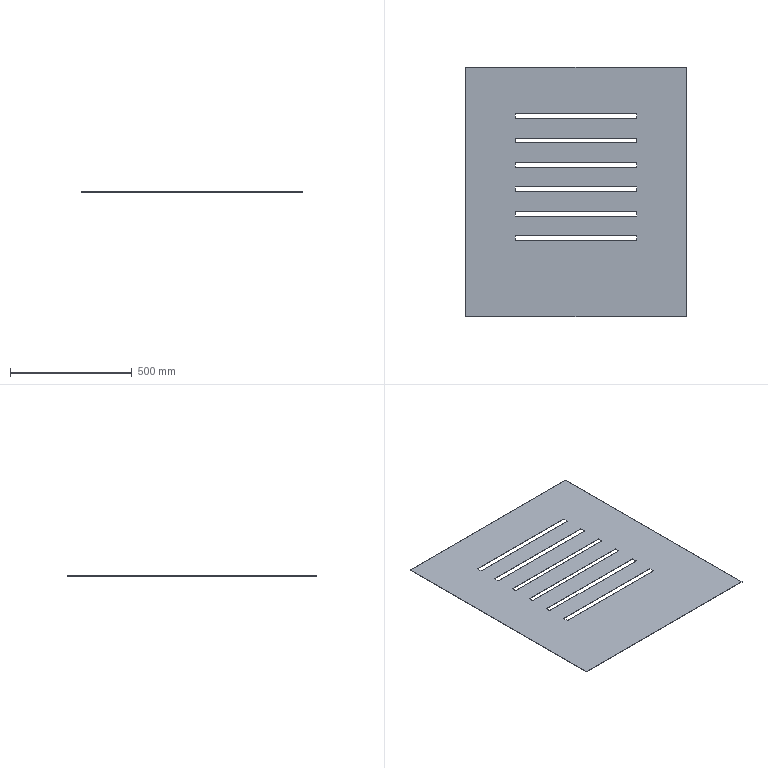Part | SolidWorks | features FlatPattern 1, SMBaseFlange 1, SheetMetal 1 | 1 solid | 30 faces | box 904 x 1022 x 1.5 mm | volume 1296374 mm3 | plane 30
STEP:
#1=CARTESIAN_POINT('',(-452.,0.,1.5));
#2=VERTEX_POINT('',#1);
#3=CARTESIAN_POINT('',(-452.,-1022.4,1.5));
#4=VERTEX_POINT('',#3);
#5=CARTESIAN_POINT('',(-452.,0.,1.5));
#6=DIRECTION('',(0.,-1.,0.));
#7=VECTOR('',#6,1000.);
#8=LINE('',#5,#7);
#9=EDGE_CURVE('',#2,#4,#8,.T.);
#10=ORIENTED_EDGE('',*,*,#9,.T.);
#11=CARTESIAN_POINT('',(452.,-1022.4,1.5));
#12=VERTEX_POINT('',#11);
#13=CARTESIAN_POINT('',(-452.,-1022.4,1.5));
#14=DIRECTION('',(1.,0.,0.));
#15=VECTOR('',#14,1000.);
#16=LINE('',#13,#15);
#17=EDGE_CURVE('',#4,#12,#16,.T.);
#18=ORIENTED_EDGE('',*,*,#17,.T.);
#19=CARTESIAN_POINT('',(452.,0.,1.5));
#20=VERTEX_POINT('',#19);
#21=CARTESIAN_POINT('',(452.,0.,1.5));
#22=DIRECTION('',(0.,1.,0.));
#23=VECTOR('',#22,1000.);
#24=LINE('',#21,#23);
#25=EDGE_CURVE('',#12,#20,#24,.T.);
#26=ORIENTED_EDGE('',*,*,#25,.T.);
#27=CARTESIAN_POINT('',(-452.,0.,1.5));
#28=DIRECTION('',(-1.,0.,0.));
#29=VECTOR('',#28,1000.);
#30=LINE('',#27,#29);
#31=EDGE_CURVE('',#20,#2,#30,.T.);
#32=ORIENTED_EDGE('',*,*,#31,.T.);
#33=EDGE_LOOP('',(#10,#18,#26,#32));
#34=FACE_OUTER_BOUND('',#33,.T.);
#35=CARTESIAN_POINT('',(250.,-190.,1.5));
#36=VERTEX_POINT('',#35);
#37=CARTESIAN_POINT('',(-250.,-190.,1.5));
#38=VERTEX_POINT('',#37);
#39=CARTESIAN_POINT('',(-250.,-190.,1.5));
#40=DIRECTION('',(-1.,0.,0.));
#41=VECTOR('',#40,1000.);
#42=LINE('',#39,#41);
#43=EDGE_CURVE('',#36,#38,#42,.T.);
#44=ORIENTED_EDGE('',*,*,#43,.F.);
#45=CARTESIAN_POINT('',(250.,-210.,1.5));
#46=VERTEX_POINT('',#45);
#47=CARTESIAN_POINT('',(250.,-210.,1.5));
#48=DIRECTION('',(0.,1.,0.));
#49=VECTOR('',#48,1000.);
#50=LINE('',#47,#49);
#51=EDGE_CURVE('',#46,#36,#50,.T.);
#52=ORIENTED_EDGE('',*,*,#51,.F.);
#53=CARTESIAN_POINT('',(-250.,-210.,1.5));
#54=VERTEX_POINT('',#53);
#55=CARTESIAN_POINT('',(-250.,-210.,1.5));
#56=DIRECTION('',(1.,0.,0.));
#57=VECTOR('',#56,1000.);
#58=LINE('',#55,#57);
#59=EDGE_CURVE('',#54,#46,#58,.T.);
#60=ORIENTED_EDGE('',*,*,#59,.F.);
#61=CARTESIAN_POINT('',(-250.,-210.,1.5));
#62=DIRECTION('',(0.,-1.,0.));
#63=VECTOR('',#62,1000.);
#64=LINE('',#61,#63);
#65=EDGE_CURVE('',#38,#54,#64,.T.);
#66=ORIENTED_EDGE('',*,*,#65,.F.);
#67=EDGE_LOOP('',(#44,#52,#60,#66));
#68=FACE_BOUND('',#67,.T.);
#69=CARTESIAN_POINT('',(250.,-290.,1.5));
#70=VERTEX_POINT('',#69);
#71=CARTESIAN_POINT('',(-250.,-290.,1.5));
#72=VERTEX_POINT('',#71);
#73=CARTESIAN_POINT('',(-250.,-290.,1.5));
#74=DIRECTION('',(-1.,0.,0.));
#75=VECTOR('',#74,1000.);
#76=LINE('',#73,#75);
#77=EDGE_CURVE('',#70,#72,#76,.T.);
#78=ORIENTED_EDGE('',*,*,#77,.F.);
#79=CARTESIAN_POINT('',(250.,-310.,1.5));
#80=VERTEX_POINT('',#79);
#81=CARTESIAN_POINT('',(250.,-310.,1.5));
#82=DIRECTION('',(0.,1.,0.));
#83=VECTOR('',#82,1000.);
#84=LINE('',#81,#83);
#85=EDGE_CURVE('',#80,#70,#84,.T.);
#86=ORIENTED_EDGE('',*,*,#85,.F.);
#87=CARTESIAN_POINT('',(-250.,-310.,1.5));
#88=VERTEX_POINT('',#87);
#89=CARTESIAN_POINT('',(-250.,-310.,1.5));
#90=DIRECTION('',(1.,0.,0.));
#91=VECTOR('',#90,1000.);
#92=LINE('',#89,#91);
#93=EDGE_CURVE('',#88,#80,#92,.T.);
#94=ORIENTED_EDGE('',*,*,#93,.F.);
#95=CARTESIAN_POINT('',(-250.,-310.,1.5));
#96=DIRECTION('',(0.,-1.,0.));
#97=VECTOR('',#96,1000.);
#98=LINE('',#95,#97);
#99=EDGE_CURVE('',#72,#88,#98,.T.);
#100=ORIENTED_EDGE('',*,*,#99,.F.);
#101=EDGE_LOOP('',(#78,#86,#94,#100));
#102=FACE_BOUND('',#101,.T.);
#103=CARTESIAN_POINT('',(250.,-390.,1.5));
#104=VERTEX_POINT('',#103);
#105=CARTESIAN_POINT('',(-250.,-390.,1.5));
#106=VERTEX_POINT('',#105);
#107=CARTESIAN_POINT('',(-250.,-390.,1.5));
#108=DIRECTION('',(-1.,0.,0.));
#109=VECTOR('',#108,1000.);
#110=LINE('',#107,#109);
#111=EDGE_CURVE('',#104,#106,#110,.T.);
#112=ORIENTED_EDGE('',*,*,#111,.F.);
#113=CARTESIAN_POINT('',(250.,-410.,1.5));
#114=VERTEX_POINT('',#113);
#115=CARTESIAN_POINT('',(250.,-410.,1.5));
#116=DIRECTION('',(0.,1.,0.));
#117=VECTOR('',#116,1000.);
#118=LINE('',#115,#117);
#119=EDGE_CURVE('',#114,#104,#118,.T.);
#120=ORIENTED_EDGE('',*,*,#119,.F.);
#121=CARTESIAN_POINT('',(-250.,-410.,1.5));
#122=VERTEX_POINT('',#121);
#123=CARTESIAN_POINT('',(-250.,-410.,1.5));
#124=DIRECTION('',(1.,0.,0.));
#125=VECTOR('',#124,1000.);
#126=LINE('',#123,#125);
#127=EDGE_CURVE('',#122,#114,#126,.T.);
#128=ORIENTED_EDGE('',*,*,#127,.F.);
#129=CARTESIAN_POINT('',(-250.,-410.,1.5));
#130=DIRECTION('',(0.,-1.,0.));
#131=VECTOR('',#130,1000.);
#132=LINE('',#129,#131);
#133=EDGE_CURVE('',#106,#122,#132,.T.);
#134=ORIENTED_EDGE('',*,*,#133,.F.);
#135=EDGE_LOOP('',(#112,#120,#128,#134));
#136=FACE_BOUND('',#135,.T.);
#137=CARTESIAN_POINT('',(250.,-490.,1.5));
#138=VERTEX_POINT('',#137);
#139=CARTESIAN_POINT('',(-250.,-490.,1.5));
#140=VERTEX_POINT('',#139);
#141=CARTESIAN_POINT('',(-250.,-490.,1.5));
#142=DIRECTION('',(-1.,0.,0.));
#143=VECTOR('',#142,1000.);
#144=LINE('',#141,#143);
#145=EDGE_CURVE('',#138,#140,#144,.T.);
#146=ORIENTED_EDGE('',*,*,#145,.F.);
#147=CARTESIAN_POINT('',(250.,-510.,1.5));
#148=VERTEX_POINT('',#147);
#149=CARTESIAN_POINT('',(250.,-510.,1.5));
#150=DIRECTION('',(0.,1.,0.));
#151=VECTOR('',#150,1000.);
#152=LINE('',#149,#151);
#153=EDGE_CURVE('',#148,#138,#152,.T.);
#154=ORIENTED_EDGE('',*,*,#153,.F.);
#155=CARTESIAN_POINT('',(-250.,-510.,1.5));
#156=VERTEX_POINT('',#155);
#157=CARTESIAN_POINT('',(-250.,-510.,1.5));
#158=DIRECTION('',(1.,0.,0.));
#159=VECTOR('',#158,1000.);
#160=LINE('',#157,#159);
#161=EDGE_CURVE('',#156,#148,#160,.T.);
#162=ORIENTED_EDGE('',*,*,#161,.F.);
#163=CARTESIAN_POINT('',(-250.,-510.,1.5));
#164=DIRECTION('',(0.,-1.,0.));
#165=VECTOR('',#164,1000.);
#166=LINE('',#163,#165);
#167=EDGE_CURVE('',#140,#156,#166,.T.);
#168=ORIENTED_EDGE('',*,*,#167,.F.);
#169=EDGE_LOOP('',(#146,#154,#162,#168));
#170=FACE_BOUND('',#169,.T.);
#171=CARTESIAN_POINT('',(250.,-590.,1.5));
#172=VERTEX_POINT('',#171);
#173=CARTESIAN_POINT('',(-250.,-590.,1.5));
#174=VERTEX_POINT('',#173);
#175=CARTESIAN_POINT('',(-250.,-590.,1.5));
#176=DIRECTION('',(-1.,0.,0.));
#177=VECTOR('',#176,1000.);
#178=LINE('',#175,#177);
#179=EDGE_CURVE('',#172,#174,#178,.T.);
#180=ORIENTED_EDGE('',*,*,#179,.F.);
#181=CARTESIAN_POINT('',(250.,-610.,1.5));
#182=VERTEX_POINT('',#181);
#183=CARTESIAN_POINT('',(250.,-610.,1.5));
#184=DIRECTION('',(0.,1.,0.));
#185=VECTOR('',#184,1000.);
#186=LINE('',#183,#185);
#187=EDGE_CURVE('',#182,#172,#186,.T.);
#188=ORIENTED_EDGE('',*,*,#187,.F.);
#189=CARTESIAN_POINT('',(-250.,-610.,1.5));
#190=VERTEX_POINT('',#189);
#191=CARTESIAN_POINT('',(-250.,-610.,1.5));
#192=DIRECTION('',(1.,0.,0.));
#193=VECTOR('',#192,1000.);
#194=LINE('',#191,#193);
#195=EDGE_CURVE('',#190,#182,#194,.T.);
#196=ORIENTED_EDGE('',*,*,#195,.F.);
#197=CARTESIAN_POINT('',(-250.,-610.,1.5));
#198=DIRECTION('',(0.,-1.,0.));
#199=VECTOR('',#198,1000.);
#200=LINE('',#197,#199);
#201=EDGE_CURVE('',#174,#190,#200,.T.);
#202=ORIENTED_EDGE('',*,*,#201,.F.);
#203=EDGE_LOOP('',(#180,#188,#196,#202));
#204=FACE_BOUND('',#203,.T.);
#205=CARTESIAN_POINT('',(250.,-690.,1.5));
#206=VERTEX_POINT('',#205);
#207=CARTESIAN_POINT('',(-250.,-690.,1.5));
#208=VERTEX_POINT('',#207);
#209=CARTESIAN_POINT('',(-250.,-690.,1.5));
#210=DIRECTION('',(-1.,0.,0.));
#211=VECTOR('',#210,1000.);
#212=LINE('',#209,#211);
#213=EDGE_CURVE('',#206,#208,#212,.T.);
#214=ORIENTED_EDGE('',*,*,#213,.F.);
#215=CARTESIAN_POINT('',(250.,-710.,1.5));
#216=VERTEX_POINT('',#215);
#217=CARTESIAN_POINT('',(250.,-710.,1.5));
#218=DIRECTION('',(0.,1.,0.));
#219=VECTOR('',#218,1000.);
#220=LINE('',#217,#219);
#221=EDGE_CURVE('',#216,#206,#220,.T.);
#222=ORIENTED_EDGE('',*,*,#221,.F.);
#223=CARTESIAN_POINT('',(-250.,-710.,1.5));
#224=VERTEX_POINT('',#223);
#225=CARTESIAN_POINT('',(-250.,-710.,1.5));
#226=DIRECTION('',(1.,0.,0.));
#227=VECTOR('',#226,1000.);
#228=LINE('',#225,#227);
#229=EDGE_CURVE('',#224,#216,#228,.T.);
#230=ORIENTED_EDGE('',*,*,#229,.F.);
#231=CARTESIAN_POINT('',(-250.,-710.,1.5));
#232=DIRECTION('',(0.,-1.,0.));
#233=VECTOR('',#232,1000.);
#234=LINE('',#231,#233);
#235=EDGE_CURVE('',#208,#224,#234,.T.);
#236=ORIENTED_EDGE('',*,*,#235,.F.);
#237=EDGE_LOOP('',(#214,#222,#230,#236));
#238=FACE_BOUND('',#237,.T.);
#239=CARTESIAN_POINT('',(0.,0.,1.5));
#240=DIRECTION('',(0.,0.,1.));
#241=DIRECTION('',(1.,0.,0.));
#242=AXIS2_PLACEMENT_3D('',#239,#240,#241);
#243=PLANE('',#242);
#244=ADVANCED_FACE('',(#34,#68,#102,#136,#170,#204,#238),#243,.T.);
#245=CARTESIAN_POINT('',(250.,-610.,0.));
#246=VERTEX_POINT('',#245);
#247=CARTESIAN_POINT('',(250.,-590.,0.));
#248=VERTEX_POINT('',#247);
#249=CARTESIAN_POINT('',(250.,-610.,0.));
#250=DIRECTION('',(0.,1.,0.));
#251=VECTOR('',#250,1000.);
#252=LINE('',#249,#251);
#253=EDGE_CURVE('',#246,#248,#252,.T.);
#254=ORIENTED_EDGE('',*,*,#253,.T.);
#255=CARTESIAN_POINT('',(-250.,-590.,0.));
#256=VERTEX_POINT('',#255);
#257=CARTESIAN_POINT('',(-250.,-590.,0.));
#258=DIRECTION('',(-1.,0.,0.));
#259=VECTOR('',#258,1000.);
#260=LINE('',#257,#259);
#261=EDGE_CURVE('',#248,#256,#260,.T.);
#262=ORIENTED_EDGE('',*,*,#261,.T.);
#263=CARTESIAN_POINT('',(-250.,-610.,0.));
#264=VERTEX_POINT('',#263);
#265=CARTESIAN_POINT('',(-250.,-610.,0.));
#266=DIRECTION('',(0.,-1.,0.));
#267=VECTOR('',#266,1000.);
#268=LINE('',#265,#267);
#269=EDGE_CURVE('',#256,#264,#268,.T.);
#270=ORIENTED_EDGE('',*,*,#269,.T.);
#271=CARTESIAN_POINT('',(-250.,-610.,0.));
#272=DIRECTION('',(1.,0.,0.));
#273=VECTOR('',#272,1000.);
#274=LINE('',#271,#273);
#275=EDGE_CURVE('',#264,#246,#274,.T.);
#276=ORIENTED_EDGE('',*,*,#275,.T.);
#277=EDGE_LOOP('',(#254,#262,#270,#276));
#278=FACE_BOUND('',#277,.T.);
#279=CARTESIAN_POINT('',(250.,-410.,0.));
#280=VERTEX_POINT('',#279);
#281=CARTESIAN_POINT('',(250.,-390.,0.));
#282=VERTEX_POINT('',#281);
#283=CARTESIAN_POINT('',(250.,-410.,0.));
#284=DIRECTION('',(0.,1.,0.));
#285=VECTOR('',#284,1000.);
#286=LINE('',#283,#285);
#287=EDGE_CURVE('',#280,#282,#286,.T.);
#288=ORIENTED_EDGE('',*,*,#287,.T.);
#289=CARTESIAN_POINT('',(-250.,-390.,0.));
#290=VERTEX_POINT('',#289);
#291=CARTESIAN_POINT('',(-250.,-390.,0.));
#292=DIRECTION('',(-1.,0.,0.));
#293=VECTOR('',#292,1000.);
#294=LINE('',#291,#293);
#295=EDGE_CURVE('',#282,#290,#294,.T.);
#296=ORIENTED_EDGE('',*,*,#295,.T.);
#297=CARTESIAN_POINT('',(-250.,-410.,0.));
#298=VERTEX_POINT('',#297);
#299=CARTESIAN_POINT('',(-250.,-410.,0.));
#300=DIRECTION('',(0.,-1.,0.));
#301=VECTOR('',#300,1000.);
#302=LINE('',#299,#301);
#303=EDGE_CURVE('',#290,#298,#302,.T.);
#304=ORIENTED_EDGE('',*,*,#303,.T.);
#305=CARTESIAN_POINT('',(-250.,-410.,0.));
#306=DIRECTION('',(1.,0.,0.));
#307=VECTOR('',#306,1000.);
#308=LINE('',#305,#307);
#309=EDGE_CURVE('',#298,#280,#308,.T.);
#310=ORIENTED_EDGE('',*,*,#309,.T.);
#311=EDGE_LOOP('',(#288,#296,#304,#310));
#312=FACE_BOUND('',#311,.T.);
#313=CARTESIAN_POINT('',(250.,-210.,0.));
#314=VERTEX_POINT('',#313);
#315=CARTESIAN_POINT('',(250.,-190.,0.));
#316=VERTEX_POINT('',#315);
#317=CARTESIAN_POINT('',(250.,-210.,0.));
#318=DIRECTION('',(0.,1.,0.));
#319=VECTOR('',#318,1000.);
#320=LINE('',#317,#319);
#321=EDGE_CURVE('',#314,#316,#320,.T.);
#322=ORIENTED_EDGE('',*,*,#321,.T.);
#323=CARTESIAN_POINT('',(-250.,-190.,0.));
#324=VERTEX_POINT('',#323);
#325=CARTESIAN_POINT('',(-250.,-190.,0.));
#326=DIRECTION('',(-1.,0.,0.));
#327=VECTOR('',#326,1000.);
#328=LINE('',#325,#327);
#329=EDGE_CURVE('',#316,#324,#328,.T.);
#330=ORIENTED_EDGE('',*,*,#329,.T.);
#331=CARTESIAN_POINT('',(-250.,-210.,0.));
#332=VERTEX_POINT('',#331);
#333=CARTESIAN_POINT('',(-250.,-210.,0.));
#334=DIRECTION('',(0.,-1.,0.));
#335=VECTOR('',#334,1000.);
#336=LINE('',#333,#335);
#337=EDGE_CURVE('',#324,#332,#336,.T.);
#338=ORIENTED_EDGE('',*,*,#337,.T.);
#339=CARTESIAN_POINT('',(-250.,-210.,0.));
#340=DIRECTION('',(1.,0.,0.));
#341=VECTOR('',#340,1000.);
#342=LINE('',#339,#341);
#343=EDGE_CURVE('',#332,#314,#342,.T.);
#344=ORIENTED_EDGE('',*,*,#343,.T.);
#345=EDGE_LOOP('',(#322,#330,#338,#344));
#346=FACE_BOUND('',#345,.T.);
#347=CARTESIAN_POINT('',(-452.,0.,0.));
#348=VERTEX_POINT('',#347);
#349=CARTESIAN_POINT('',(-452.,-1022.4,0.));
#350=VERTEX_POINT('',#349);
#351=CARTESIAN_POINT('',(-452.,0.,0.));
#352=DIRECTION('',(0.,-1.,0.));
#353=VECTOR('',#352,1000.);
#354=LINE('',#351,#353);
#355=EDGE_CURVE('',#348,#350,#354,.T.);
#356=ORIENTED_EDGE('',*,*,#355,.F.);
#357=CARTESIAN_POINT('',(452.,0.,0.));
#358=VERTEX_POINT('',#357);
#359=CARTESIAN_POINT('',(-452.,0.,0.));
#360=DIRECTION('',(-1.,0.,0.));
#361=VECTOR('',#360,1000.);
#362=LINE('',#359,#361);
#363=EDGE_CURVE('',#358,#348,#362,.T.);
#364=ORIENTED_EDGE('',*,*,#363,.F.);
#365=CARTESIAN_POINT('',(452.,-1022.4,0.));
#366=VERTEX_POINT('',#365);
#367=CARTESIAN_POINT('',(452.,0.,0.));
#368=DIRECTION('',(0.,1.,0.));
#369=VECTOR('',#368,1000.);
#370=LINE('',#367,#369);
#371=EDGE_CURVE('',#366,#358,#370,.T.);
#372=ORIENTED_EDGE('',*,*,#371,.F.);
#373=CARTESIAN_POINT('',(-452.,-1022.4,0.));
#374=DIRECTION('',(1.,0.,0.));
#375=VECTOR('',#374,1000.);
#376=LINE('',#373,#375);
#377=EDGE_CURVE('',#350,#366,#376,.T.);
#378=ORIENTED_EDGE('',*,*,#377,.F.);
#379=EDGE_LOOP('',(#356,#364,#372,#378));
#380=FACE_OUTER_BOUND('',#379,.T.);
#381=CARTESIAN_POINT('',(250.,-310.,0.));
#382=VERTEX_POINT('',#381);
#383=CARTESIAN_POINT('',(250.,-290.,0.));
#384=VERTEX_POINT('',#383);
#385=CARTESIAN_POINT('',(250.,-310.,0.));
#386=DIRECTION('',(0.,1.,0.));
#387=VECTOR('',#386,1000.);
#388=LINE('',#385,#387);
#389=EDGE_CURVE('',#382,#384,#388,.T.);
#390=ORIENTED_EDGE('',*,*,#389,.T.);
#391=CARTESIAN_POINT('',(-250.,-290.,0.));
#392=VERTEX_POINT('',#391);
#393=CARTESIAN_POINT('',(-250.,-290.,0.));
#394=DIRECTION('',(-1.,0.,0.));
#395=VECTOR('',#394,1000.);
#396=LINE('',#393,#395);
#397=EDGE_CURVE('',#384,#392,#396,.T.);
#398=ORIENTED_EDGE('',*,*,#397,.T.);
#399=CARTESIAN_POINT('',(-250.,-310.,0.));
#400=VERTEX_POINT('',#399);
#401=CARTESIAN_POINT('',(-250.,-310.,0.));
#402=DIRECTION('',(0.,-1.,0.));
#403=VECTOR('',#402,1000.);
#404=LINE('',#401,#403);
#405=EDGE_CURVE('',#392,#400,#404,.T.);
#406=ORIENTED_EDGE('',*,*,#405,.T.);
#407=CARTESIAN_POINT('',(-250.,-310.,0.));
#408=DIRECTION('',(1.,0.,0.));
#409=VECTOR('',#408,1000.);
#410=LINE('',#407,#409);
#411=EDGE_CURVE('',#400,#382,#410,.T.);
#412=ORIENTED_EDGE('',*,*,#411,.T.);
#413=EDGE_LOOP('',(#390,#398,#406,#412));
#414=FACE_BOUND('',#413,.T.);
#415=CARTESIAN_POINT('',(250.,-510.,0.));
#416=VERTEX_POINT('',#415);
#417=CARTESIAN_POINT('',(250.,-490.,0.));
#418=VERTEX_POINT('',#417);
#419=CARTESIAN_POINT('',(250.,-510.,0.));
#420=DIRECTION('',(0.,1.,0.));
#421=VECTOR('',#420,1000.);
#422=LINE('',#419,#421);
#423=EDGE_CURVE('',#416,#418,#422,.T.);
#424=ORIENTED_EDGE('',*,*,#423,.T.);
#425=CARTESIAN_POINT('',(-250.,-490.,0.));
#426=VERTEX_POINT('',#425);
#427=CARTESIAN_POINT('',(-250.,-490.,0.));
#428=DIRECTION('',(-1.,0.,0.));
#429=VECTOR('',#428,1000.);
#430=LINE('',#427,#429);
#431=EDGE_CURVE('',#418,#426,#430,.T.);
#432=ORIENTED_EDGE('',*,*,#431,.T.);
#433=CARTESIAN_POINT('',(-250.,-510.,0.));
#434=VERTEX_POINT('',#433);
#435=CARTESIAN_POINT('',(-250.,-510.,0.));
#436=DIRECTION('',(0.,-1.,0.));
#437=VECTOR('',#436,1000.);
#438=LINE('',#435,#437);
#439=EDGE_CURVE('',#426,#434,#438,.T.);
#440=ORIENTED_EDGE('',*,*,#439,.T.);
#441=CARTESIAN_POINT('',(-250.,-510.,0.));
#442=DIRECTION('',(1.,0.,0.));
#443=VECTOR('',#442,1000.);
#444=LINE('',#441,#443);
#445=EDGE_CURVE('',#434,#416,#444,.T.);
#446=ORIENTED_EDGE('',*,*,#445,.T.);
#447=EDGE_LOOP('',(#424,#432,#440,#446));
#448=FACE_BOUND('',#447,.T.);
#449=CARTESIAN_POINT('',(250.,-710.,0.));
#450=VERTEX_POINT('',#449);
#451=CARTESIAN_POINT('',(250.,-690.,0.));
#452=VERTEX_POINT('',#451);
#453=CARTESIAN_POINT('',(250.,-710.,0.));
#454=DIRECTION('',(0.,1.,0.));
#455=VECTOR('',#454,1000.);
#456=LINE('',#453,#455);
#457=EDGE_CURVE('',#450,#452,#456,.T.);
#458=ORIENTED_EDGE('',*,*,#457,.T.);
#459=CARTESIAN_POINT('',(-250.,-690.,0.));
#460=VERTEX_POINT('',#459);
#461=CARTESIAN_POINT('',(-250.,-690.,0.));
#462=DIRECTION('',(-1.,0.,0.));
#463=VECTOR('',#462,1000.);
#464=LINE('',#461,#463);
#465=EDGE_CURVE('',#452,#460,#464,.T.);
#466=ORIENTED_EDGE('',*,*,#465,.T.);
#467=CARTESIAN_POINT('',(-250.,-710.,0.));
#468=VERTEX_POINT('',#467);
#469=CARTESIAN_POINT('',(-250.,-710.,0.));
#470=DIRECTION('',(0.,-1.,0.));
#471=VECTOR('',#470,1000.);
#472=LINE('',#469,#471);
#473=EDGE_CURVE('',#460,#468,#472,.T.);
#474=ORIENTED_EDGE('',*,*,#473,.T.);
#475=CARTESIAN_POINT('',(-250.,-710.,0.));
#476=DIRECTION('',(1.,0.,0.));
#477=VECTOR('',#476,1000.);
#478=LINE('',#475,#477);
#479=EDGE_CURVE('',#468,#450,#478,.T.);
#480=ORIENTED_EDGE('',*,*,#479,.T.);
#481=EDGE_LOOP('',(#458,#466,#474,#480));
#482=FACE_BOUND('',#481,.T.);
#483=CARTESIAN_POINT('',(0.,0.,0.));
#484=DIRECTION('',(0.,0.,1.));
#485=DIRECTION('',(1.,0.,0.));
#486=AXIS2_PLACEMENT_3D('',#483,#484,#485);
#487=PLANE('',#486);
#488=ADVANCED_FACE('',(#278,#312,#346,#380,#414,#448,#482),#487,.F.);
#489=ORIENTED_EDGE('',*,*,#355,.T.);
#490=CARTESIAN_POINT('',(-452.,-1022.4,1.5));
#491=DIRECTION('',(0.,0.,-1.));
#492=VECTOR('',#491,1000.);
#493=LINE('',#490,#492);
#494=EDGE_CURVE('',#4,#350,#493,.T.);
#495=ORIENTED_EDGE('',*,*,#494,.F.);
#496=ORIENTED_EDGE('',*,*,#9,.F.);
#497=CARTESIAN_POINT('',(-452.,0.,1.5));
#498=DIRECTION('',(0.,0.,-1.));
#499=VECTOR('',#498,1000.);
#500=LINE('',#497,#499);
#501=EDGE_CURVE('',#2,#348,#500,.T.);
#502=ORIENTED_EDGE('',*,*,#501,.T.);
#503=EDGE_LOOP('',(#489,#495,#496,#502));
#504=FACE_OUTER_BOUND('',#503,.T.);
#505=CARTESIAN_POINT('',(-452.,0.,1.5));
#506=DIRECTION('',(1.,0.,0.));
#507=DIRECTION('',(0.,1.,0.));
#508=AXIS2_PLACEMENT_3D('',#505,#506,#507);
#509=PLANE('',#508);
#510=ADVANCED_FACE('',(#504),#509,.F.);
#511=ORIENTED_EDGE('',*,*,#377,.T.);
#512=CARTESIAN_POINT('',(452.,-1022.4,1.5));
#513=DIRECTION('',(0.,0.,-1.));
#514=VECTOR('',#513,1000.);
#515=LINE('',#512,#514);
#516=EDGE_CURVE('',#12,#366,#515,.T.);
#517=ORIENTED_EDGE('',*,*,#516,.F.);
#518=ORIENTED_EDGE('',*,*,#17,.F.);
#519=ORIENTED_EDGE('',*,*,#494,.T.);
#520=EDGE_LOOP('',(#511,#517,#518,#519));
#521=FACE_OUTER_BOUND('',#520,.T.);
#522=CARTESIAN_POINT('',(-452.,-1022.4,1.5));
#523=DIRECTION('',(0.,1.,0.));
#524=DIRECTION('',(0.,0.,1.));
#525=AXIS2_PLACEMENT_3D('',#522,#523,#524);
#526=PLANE('',#525);
#527=ADVANCED_FACE('',(#521),#526,.F.);
#528=ORIENTED_EDGE('',*,*,#371,.T.);
#529=CARTESIAN_POINT('',(452.,0.,1.5));
#530=DIRECTION('',(0.,0.,-1.));
#531=VECTOR('',#530,1000.);
#532=LINE('',#529,#531);
#533=EDGE_CURVE('',#20,#358,#532,.T.);
#534=ORIENTED_EDGE('',*,*,#533,.F.);
#535=ORIENTED_EDGE('',*,*,#25,.F.);
#536=ORIENTED_EDGE('',*,*,#516,.T.);
#537=EDGE_LOOP('',(#528,#534,#535,#536));
#538=FACE_OUTER_BOUND('',#537,.T.);
#539=CARTESIAN_POINT('',(452.,0.,1.5));
#540=DIRECTION('',(-1.,0.,0.));
#541=DIRECTION('',(0.,0.,1.));
#542=AXIS2_PLACEMENT_3D('',#539,#540,#541);
#543=PLANE('',#542);
#544=ADVANCED_FACE('',(#538),#543,.F.);
#545=ORIENTED_EDGE('',*,*,#363,.T.);
#546=ORIENTED_EDGE('',*,*,#501,.F.);
#547=ORIENTED_EDGE('',*,*,#31,.F.);
#548=ORIENTED_EDGE('',*,*,#533,.T.);
#549=EDGE_LOOP('',(#545,#546,#547,#548));
#550=FACE_OUTER_BOUND('',#549,.T.);
#551=CARTESIAN_POINT('',(-452.,0.,1.5));
#552=DIRECTION('',(0.,-1.,0.));
#553=DIRECTION('',(0.,0.,-1.));
#554=AXIS2_PLACEMENT_3D('',#551,#552,#553);
#555=PLANE('',#554);
#556=ADVANCED_FACE('',(#550),#555,.F.);
#557=ORIENTED_EDGE('',*,*,#321,.F.);
#558=CARTESIAN_POINT('',(250.,-210.,1.5));
#559=DIRECTION('',(0.,0.,-1.));
#560=VECTOR('',#559,1000.);
#561=LINE('',#558,#560);
#562=EDGE_CURVE('',#46,#314,#561,.T.);
#563=ORIENTED_EDGE('',*,*,#562,.F.);
#564=ORIENTED_EDGE('',*,*,#51,.T.);
#565=CARTESIAN_POINT('',(250.,-190.,1.5));
#566=DIRECTION('',(0.,0.,-1.));
#567=VECTOR('',#566,1000.);
#568=LINE('',#565,#567);
#569=EDGE_CURVE('',#36,#316,#568,.T.);
#570=ORIENTED_EDGE('',*,*,#569,.T.);
#571=EDGE_LOOP('',(#557,#563,#564,#570));
#572=FACE_OUTER_BOUND('',#571,.T.);
#573=CARTESIAN_POINT('',(250.,-210.,1.5));
#574=DIRECTION('',(-1.,0.,0.));
#575=DIRECTION('',(0.,-1.,0.));
#576=AXIS2_PLACEMENT_3D('',#573,#574,#575);
#577=PLANE('',#576);
#578=ADVANCED_FACE('',(#572),#577,.T.);
#579=ORIENTED_EDGE('',*,*,#329,.F.);
#580=ORIENTED_EDGE('',*,*,#569,.F.);
#581=ORIENTED_EDGE('',*,*,#43,.T.);
#582=CARTESIAN_POINT('',(-250.,-190.,1.5));
#583=DIRECTION('',(0.,0.,-1.));
#584=VECTOR('',#583,1000.);
#585=LINE('',#582,#584);
#586=EDGE_CURVE('',#38,#324,#585,.T.);
#587=ORIENTED_EDGE('',*,*,#586,.T.);
#588=EDGE_LOOP('',(#579,#580,#581,#587));
#589=FACE_OUTER_BOUND('',#588,.T.);
#590=CARTESIAN_POINT('',(-250.,-190.,1.5));
#591=DIRECTION('',(0.,-1.,0.));
#592=DIRECTION('',(1.,0.,0.));
#593=AXIS2_PLACEMENT_3D('',#590,#591,#592);
#594=PLANE('',#593);
#595=ADVANCED_FACE('',(#589),#594,.T.);
#596=ORIENTED_EDGE('',*,*,#337,.F.);
#597=ORIENTED_EDGE('',*,*,#586,.F.);
#598=ORIENTED_EDGE('',*,*,#65,.T.);
#599=CARTESIAN_POINT('',(-250.,-210.,1.5));
#600=DIRECTION('',(0.,0.,-1.));
#601=VECTOR('',#600,1000.);
#602=LINE('',#599,#601);
#603=EDGE_CURVE('',#54,#332,#602,.T.);
#604=ORIENTED_EDGE('',*,*,#603,.T.);
#605=EDGE_LOOP('',(#596,#597,#598,#604));
#606=FACE_OUTER_BOUND('',#605,.T.);
#607=CARTESIAN_POINT('',(-250.,-210.,1.5));
#608=DIRECTION('',(1.,0.,0.));
#609=DIRECTION('',(0.,0.,-1.));
#610=AXIS2_PLACEMENT_3D('',#607,#608,#609);
#611=PLANE('',#610);
#612=ADVANCED_FACE('',(#606),#611,.T.);
#613=ORIENTED_EDGE('',*,*,#343,.F.);
#614=ORIENTED_EDGE('',*,*,#603,.F.);
#615=ORIENTED_EDGE('',*,*,#59,.T.);
#616=ORIENTED_EDGE('',*,*,#562,.T.);
#617=EDGE_LOOP('',(#613,#614,#615,#616));
#618=FACE_OUTER_BOUND('',#617,.T.);
#619=CARTESIAN_POINT('',(-250.,-210.,1.5));
#620=DIRECTION('',(0.,1.,0.));
#621=DIRECTION('',(0.,0.,1.));
#622=AXIS2_PLACEMENT_3D('',#619,#620,#621);
#623=PLANE('',#622);
#624=ADVANCED_FACE('',(#618),#623,.T.);
#625=ORIENTED_EDGE('',*,*,#389,.F.);
#626=CARTESIAN_POINT('',(250.,-310.,1.5));
#627=DIRECTION('',(0.,0.,-1.));
#628=VECTOR('',#627,1000.);
#629=LINE('',#626,#628);
#630=EDGE_CURVE('',#80,#382,#629,.T.);
#631=ORIENTED_EDGE('',*,*,#630,.F.);
#632=ORIENTED_EDGE('',*,*,#85,.T.);
#633=CARTESIAN_POINT('',(250.,-290.,1.5));
#634=DIRECTION('',(0.,0.,-1.));
#635=VECTOR('',#634,1000.);
#636=LINE('',#633,#635);
#637=EDGE_CURVE('',#70,#384,#636,.T.);
#638=ORIENTED_EDGE('',*,*,#637,.T.);
#639=EDGE_LOOP('',(#625,#631,#632,#638));
#640=FACE_OUTER_BOUND('',#639,.T.);
#641=CARTESIAN_POINT('',(250.,-310.,1.5));
#642=DIRECTION('',(-1.,0.,0.));
#643=DIRECTION('',(0.,-1.,0.));
#644=AXIS2_PLACEMENT_3D('',#641,#642,#643);
#645=PLANE('',#644);
#646=ADVANCED_FACE('',(#640),#645,.T.);
#647=ORIENTED_EDGE('',*,*,#397,.F.);
#648=ORIENTED_EDGE('',*,*,#637,.F.);
#649=ORIENTED_EDGE('',*,*,#77,.T.);
#650=CARTESIAN_POINT('',(-250.,-290.,1.5));
#651=DIRECTION('',(0.,0.,-1.));
#652=VECTOR('',#651,1000.);
#653=LINE('',#650,#652);
#654=EDGE_CURVE('',#72,#392,#653,.T.);
#655=ORIENTED_EDGE('',*,*,#654,.T.);
#656=EDGE_LOOP('',(#647,#648,#649,#655));
#657=FACE_OUTER_BOUND('',#656,.T.);
#658=CARTESIAN_POINT('',(-250.,-290.,1.5));
#659=DIRECTION('',(0.,-1.,0.));
#660=DIRECTION('',(0.,0.,-1.));
#661=AXIS2_PLACEMENT_3D('',#658,#659,#660);
#662=PLANE('',#661);
#663=ADVANCED_FACE('',(#657),#662,.T.);
#664=ORIENTED_EDGE('',*,*,#405,.F.);
#665=ORIENTED_EDGE('',*,*,#654,.F.);
#666=ORIENTED_EDGE('',*,*,#99,.T.);
#667=CARTESIAN_POINT('',(-250.,-310.,1.5));
#668=DIRECTION('',(0.,0.,-1.));
#669=VECTOR('',#668,1000.);
#670=LINE('',#667,#669);
#671=EDGE_CURVE('',#88,#400,#670,.T.);
#672=ORIENTED_EDGE('',*,*,#671,.T.);
#673=EDGE_LOOP('',(#664,#665,#666,#672));
#674=FACE_OUTER_BOUND('',#673,.T.);
#675=CARTESIAN_POINT('',(-250.,-310.,1.5));
#676=DIRECTION('',(1.,0.,0.));
#677=DIRECTION('',(0.,0.,-1.));
#678=AXIS2_PLACEMENT_3D('',#675,#676,#677);
#679=PLANE('',#678);
#680=ADVANCED_FACE('',(#674),#679,.T.);
#681=ORIENTED_EDGE('',*,*,#411,.F.);
#682=ORIENTED_EDGE('',*,*,#671,.F.);
#683=ORIENTED_EDGE('',*,*,#93,.T.);
#684=ORIENTED_EDGE('',*,*,#630,.T.);
#685=EDGE_LOOP('',(#681,#682,#683,#684));
#686=FACE_OUTER_BOUND('',#685,.T.);
#687=CARTESIAN_POINT('',(-250.,-310.,1.5));
#688=DIRECTION('',(0.,1.,0.));
#689=DIRECTION('',(0.,0.,1.));
#690=AXIS2_PLACEMENT_3D('',#687,#688,#689);
#691=PLANE('',#690);
#692=ADVANCED_FACE('',(#686),#691,.T.);
#693=ORIENTED_EDGE('',*,*,#287,.F.);
#694=CARTESIAN_POINT('',(250.,-410.,1.5));
#695=DIRECTION('',(0.,0.,-1.));
#696=VECTOR('',#695,1000.);
#697=LINE('',#694,#696);
#698=EDGE_CURVE('',#114,#280,#697,.T.);
#699=ORIENTED_EDGE('',*,*,#698,.F.);
#700=ORIENTED_EDGE('',*,*,#119,.T.);
#701=CARTESIAN_POINT('',(250.,-390.,1.5));
#702=DIRECTION('',(0.,0.,-1.));
#703=VECTOR('',#702,1000.);
#704=LINE('',#701,#703);
#705=EDGE_CURVE('',#104,#282,#704,.T.);
#706=ORIENTED_EDGE('',*,*,#705,.T.);
#707=EDGE_LOOP('',(#693,#699,#700,#706));
#708=FACE_OUTER_BOUND('',#707,.T.);
#709=CARTESIAN_POINT('',(250.,-410.,1.5));
#710=DIRECTION('',(-1.,0.,0.));
#711=DIRECTION('',(0.,-1.,0.));
#712=AXIS2_PLACEMENT_3D('',#709,#710,#711);
#713=PLANE('',#712);
#714=ADVANCED_FACE('',(#708),#713,.T.);
#715=ORIENTED_EDGE('',*,*,#295,.F.);
#716=ORIENTED_EDGE('',*,*,#705,.F.);
#717=ORIENTED_EDGE('',*,*,#111,.T.);
#718=CARTESIAN_POINT('',(-250.,-390.,1.5));
#719=DIRECTION('',(0.,0.,-1.));
#720=VECTOR('',#719,1000.);
#721=LINE('',#718,#720);
#722=EDGE_CURVE('',#106,#290,#721,.T.);
#723=ORIENTED_EDGE('',*,*,#722,.T.);
#724=EDGE_LOOP('',(#715,#716,#717,#723));
#725=FACE_OUTER_BOUND('',#724,.T.);
#726=CARTESIAN_POINT('',(-250.,-390.,1.5));
#727=DIRECTION('',(0.,-1.,0.));
#728=DIRECTION('',(1.,0.,0.));
#729=AXIS2_PLACEMENT_3D('',#726,#727,#728);
#730=PLANE('',#729);
#731=ADVANCED_FACE('',(#725),#730,.T.);
#732=ORIENTED_EDGE('',*,*,#303,.F.);
#733=ORIENTED_EDGE('',*,*,#722,.F.);
#734=ORIENTED_EDGE('',*,*,#133,.T.);
#735=CARTESIAN_POINT('',(-250.,-410.,1.5));
#736=DIRECTION('',(0.,0.,-1.));
#737=VECTOR('',#736,1000.);
#738=LINE('',#735,#737);
#739=EDGE_CURVE('',#122,#298,#738,.T.);
#740=ORIENTED_EDGE('',*,*,#739,.T.);
#741=EDGE_LOOP('',(#732,#733,#734,#740));
#742=FACE_OUTER_BOUND('',#741,.T.);
#743=CARTESIAN_POINT('',(-250.,-410.,1.5));
#744=DIRECTION('',(1.,0.,0.));
#745=DIRECTION('',(0.,0.,-1.));
#746=AXIS2_PLACEMENT_3D('',#743,#744,#745);
#747=PLANE('',#746);
#748=ADVANCED_FACE('',(#742),#747,.T.);
#749=ORIENTED_EDGE('',*,*,#309,.F.);
#750=ORIENTED_EDGE('',*,*,#739,.F.);
#751=ORIENTED_EDGE('',*,*,#127,.T.);
#752=ORIENTED_EDGE('',*,*,#698,.T.);
#753=EDGE_LOOP('',(#749,#750,#751,#752));
#754=FACE_OUTER_BOUND('',#753,.T.);
#755=CARTESIAN_POINT('',(-250.,-410.,1.5));
#756=DIRECTION('',(0.,1.,0.));
#757=DIRECTION('',(0.,0.,1.));
#758=AXIS2_PLACEMENT_3D('',#755,#756,#757);
#759=PLANE('',#758);
#760=ADVANCED_FACE('',(#754),#759,.T.);
#761=ORIENTED_EDGE('',*,*,#423,.F.);
#762=CARTESIAN_POINT('',(250.,-510.,1.5));
#763=DIRECTION('',(0.,0.,-1.));
#764=VECTOR('',#763,1000.);
#765=LINE('',#762,#764);
#766=EDGE_CURVE('',#148,#416,#765,.T.);
#767=ORIENTED_EDGE('',*,*,#766,.F.);
#768=ORIENTED_EDGE('',*,*,#153,.T.);
#769=CARTESIAN_POINT('',(250.,-490.,1.5));
#770=DIRECTION('',(0.,0.,-1.));
#771=VECTOR('',#770,1000.);
#772=LINE('',#769,#771);
#773=EDGE_CURVE('',#138,#418,#772,.T.);
#774=ORIENTED_EDGE('',*,*,#773,.T.);
#775=EDGE_LOOP('',(#761,#767,#768,#774));
#776=FACE_OUTER_BOUND('',#775,.T.);
#777=CARTESIAN_POINT('',(250.,-510.,1.5));
#778=DIRECTION('',(-1.,0.,0.));
#779=DIRECTION('',(0.,-1.,0.));
#780=AXIS2_PLACEMENT_3D('',#777,#778,#779);
#781=PLANE('',#780);
#782=ADVANCED_FACE('',(#776),#781,.T.);
#783=ORIENTED_EDGE('',*,*,#431,.F.);
#784=ORIENTED_EDGE('',*,*,#773,.F.);
#785=ORIENTED_EDGE('',*,*,#145,.T.);
#786=CARTESIAN_POINT('',(-250.,-490.,1.5));
#787=DIRECTION('',(0.,0.,-1.));
#788=VECTOR('',#787,1000.);
#789=LINE('',#786,#788);
#790=EDGE_CURVE('',#140,#426,#789,.T.);
#791=ORIENTED_EDGE('',*,*,#790,.T.);
#792=EDGE_LOOP('',(#783,#784,#785,#791));
#793=FACE_OUTER_BOUND('',#792,.T.);
#794=CARTESIAN_POINT('',(-250.,-490.,1.5));
#795=DIRECTION('',(0.,-1.,0.));
#796=DIRECTION('',(0.,0.,-1.));
#797=AXIS2_PLACEMENT_3D('',#794,#795,#796);
#798=PLANE('',#797);
#799=ADVANCED_FACE('',(#793),#798,.T.);
#800=ORIENTED_EDGE('',*,*,#439,.F.);
#801=ORIENTED_EDGE('',*,*,#790,.F.);
#802=ORIENTED_EDGE('',*,*,#167,.T.);
#803=CARTESIAN_POINT('',(-250.,-510.,1.5));
#804=DIRECTION('',(0.,0.,-1.));
#805=VECTOR('',#804,1000.);
#806=LINE('',#803,#805);
#807=EDGE_CURVE('',#156,#434,#806,.T.);
#808=ORIENTED_EDGE('',*,*,#807,.T.);
#809=EDGE_LOOP('',(#800,#801,#802,#808));
#810=FACE_OUTER_BOUND('',#809,.T.);
#811=CARTESIAN_POINT('',(-250.,-510.,1.5));
#812=DIRECTION('',(1.,0.,0.));
#813=DIRECTION('',(0.,0.,-1.));
#814=AXIS2_PLACEMENT_3D('',#811,#812,#813);
#815=PLANE('',#814);
#816=ADVANCED_FACE('',(#810),#815,.T.);
#817=ORIENTED_EDGE('',*,*,#445,.F.);
#818=ORIENTED_EDGE('',*,*,#807,.F.);
#819=ORIENTED_EDGE('',*,*,#161,.T.);
#820=ORIENTED_EDGE('',*,*,#766,.T.);
#821=EDGE_LOOP('',(#817,#818,#819,#820));
#822=FACE_OUTER_BOUND('',#821,.T.);
#823=CARTESIAN_POINT('',(-250.,-510.,1.5));
#824=DIRECTION('',(0.,1.,0.));
#825=DIRECTION('',(0.,0.,1.));
#826=AXIS2_PLACEMENT_3D('',#823,#824,#825);
#827=PLANE('',#826);
#828=ADVANCED_FACE('',(#822),#827,.T.);
#829=ORIENTED_EDGE('',*,*,#253,.F.);
#830=CARTESIAN_POINT('',(250.,-610.,1.5));
#831=DIRECTION('',(0.,0.,-1.));
#832=VECTOR('',#831,1000.);
#833=LINE('',#830,#832);
#834=EDGE_CURVE('',#182,#246,#833,.T.);
#835=ORIENTED_EDGE('',*,*,#834,.F.);
#836=ORIENTED_EDGE('',*,*,#187,.T.);
#837=CARTESIAN_POINT('',(250.,-590.,1.5));
#838=DIRECTION('',(0.,0.,-1.));
#839=VECTOR('',#838,1000.);
#840=LINE('',#837,#839);
#841=EDGE_CURVE('',#172,#248,#840,.T.);
#842=ORIENTED_EDGE('',*,*,#841,.T.);
#843=EDGE_LOOP('',(#829,#835,#836,#842));
#844=FACE_OUTER_BOUND('',#843,.T.);
#845=CARTESIAN_POINT('',(250.,-610.,1.5));
#846=DIRECTION('',(-1.,0.,0.));
#847=DIRECTION('',(0.,-1.,0.));
#848=AXIS2_PLACEMENT_3D('',#845,#846,#847);
#849=PLANE('',#848);
#850=ADVANCED_FACE('',(#844),#849,.T.);
#851=ORIENTED_EDGE('',*,*,#261,.F.);
#852=ORIENTED_EDGE('',*,*,#841,.F.);
#853=ORIENTED_EDGE('',*,*,#179,.T.);
#854=CARTESIAN_POINT('',(-250.,-590.,1.5));
#855=DIRECTION('',(0.,0.,-1.));
#856=VECTOR('',#855,1000.);
#857=LINE('',#854,#856);
#858=EDGE_CURVE('',#174,#256,#857,.T.);
#859=ORIENTED_EDGE('',*,*,#858,.T.);
#860=EDGE_LOOP('',(#851,#852,#853,#859));
#861=FACE_OUTER_BOUND('',#860,.T.);
#862=CARTESIAN_POINT('',(-250.,-590.,1.5));
#863=DIRECTION('',(0.,-1.,0.));
#864=DIRECTION('',(0.,0.,-1.));
#865=AXIS2_PLACEMENT_3D('',#862,#863,#864);
#866=PLANE('',#865);
#867=ADVANCED_FACE('',(#861),#866,.T.);
#868=ORIENTED_EDGE('',*,*,#269,.F.);
#869=ORIENTED_EDGE('',*,*,#858,.F.);
#870=ORIENTED_EDGE('',*,*,#201,.T.);
#871=CARTESIAN_POINT('',(-250.,-610.,1.5));
#872=DIRECTION('',(0.,0.,-1.));
#873=VECTOR('',#872,1000.);
#874=LINE('',#871,#873);
#875=EDGE_CURVE('',#190,#264,#874,.T.);
#876=ORIENTED_EDGE('',*,*,#875,.T.);
#877=EDGE_LOOP('',(#868,#869,#870,#876));
#878=FACE_OUTER_BOUND('',#877,.T.);
#879=CARTESIAN_POINT('',(-250.,-610.,1.5));
#880=DIRECTION('',(1.,0.,0.));
#881=DIRECTION('',(0.,0.,-1.));
#882=AXIS2_PLACEMENT_3D('',#879,#880,#881);
#883=PLANE('',#882);
#884=ADVANCED_FACE('',(#878),#883,.T.);
#885=ORIENTED_EDGE('',*,*,#275,.F.);
#886=ORIENTED_EDGE('',*,*,#875,.F.);
#887=ORIENTED_EDGE('',*,*,#195,.T.);
#888=ORIENTED_EDGE('',*,*,#834,.T.);
#889=EDGE_LOOP('',(#885,#886,#887,#888));
#890=FACE_OUTER_BOUND('',#889,.T.);
#891=CARTESIAN_POINT('',(-250.,-610.,1.5));
#892=DIRECTION('',(0.,1.,0.));
#893=DIRECTION('',(0.,0.,1.));
#894=AXIS2_PLACEMENT_3D('',#891,#892,#893);
#895=PLANE('',#894);
#896=ADVANCED_FACE('',(#890),#895,.T.);
#897=ORIENTED_EDGE('',*,*,#457,.F.);
#898=CARTESIAN_POINT('',(250.,-710.,1.5));
#899=DIRECTION('',(0.,0.,-1.));
#900=VECTOR('',#899,1000.);
#901=LINE('',#898,#900);
#902=EDGE_CURVE('',#216,#450,#901,.T.);
#903=ORIENTED_EDGE('',*,*,#902,.F.);
#904=ORIENTED_EDGE('',*,*,#221,.T.);
#905=CARTESIAN_POINT('',(250.,-690.,1.5));
#906=DIRECTION('',(0.,0.,-1.));
#907=VECTOR('',#906,1000.);
#908=LINE('',#905,#907);
#909=EDGE_CURVE('',#206,#452,#908,.T.);
#910=ORIENTED_EDGE('',*,*,#909,.T.);
#911=EDGE_LOOP('',(#897,#903,#904,#910));
#912=FACE_OUTER_BOUND('',#911,.T.);
#913=CARTESIAN_POINT('',(250.,-710.,1.5));
#914=DIRECTION('',(-1.,0.,0.));
#915=DIRECTION('',(0.,-1.,0.));
#916=AXIS2_PLACEMENT_3D('',#913,#914,#915);
#917=PLANE('',#916);
#918=ADVANCED_FACE('',(#912),#917,.T.);
#919=ORIENTED_EDGE('',*,*,#465,.F.);
#920=ORIENTED_EDGE('',*,*,#909,.F.);
#921=ORIENTED_EDGE('',*,*,#213,.T.);
#922=CARTESIAN_POINT('',(-250.,-690.,1.5));
#923=DIRECTION('',(0.,0.,-1.));
#924=VECTOR('',#923,1000.);
#925=LINE('',#922,#924);
#926=EDGE_CURVE('',#208,#460,#925,.T.);
#927=ORIENTED_EDGE('',*,*,#926,.T.);
#928=EDGE_LOOP('',(#919,#920,#921,#927));
#929=FACE_OUTER_BOUND('',#928,.T.);
#930=CARTESIAN_POINT('',(-250.,-690.,1.5));
#931=DIRECTION('',(0.,-1.,0.));
#932=DIRECTION('',(0.,0.,-1.));
#933=AXIS2_PLACEMENT_3D('',#930,#931,#932);
#934=PLANE('',#933);
#935=ADVANCED_FACE('',(#929),#934,.T.);
#936=ORIENTED_EDGE('',*,*,#473,.F.);
#937=ORIENTED_EDGE('',*,*,#926,.F.);
#938=ORIENTED_EDGE('',*,*,#235,.T.);
#939=CARTESIAN_POINT('',(-250.,-710.,1.5));
#940=DIRECTION('',(0.,0.,-1.));
#941=VECTOR('',#940,1000.);
#942=LINE('',#939,#941);
#943=EDGE_CURVE('',#224,#468,#942,.T.);
#944=ORIENTED_EDGE('',*,*,#943,.T.);
#945=EDGE_LOOP('',(#936,#937,#938,#944));
#946=FACE_OUTER_BOUND('',#945,.T.);
#947=CARTESIAN_POINT('',(-250.,-710.,1.5));
#948=DIRECTION('',(1.,0.,0.));
#949=DIRECTION('',(0.,0.,-1.));
#950=AXIS2_PLACEMENT_3D('',#947,#948,#949);
#951=PLANE('',#950);
#952=ADVANCED_FACE('',(#946),#951,.T.);
#953=ORIENTED_EDGE('',*,*,#479,.F.);
#954=ORIENTED_EDGE('',*,*,#943,.F.);
#955=ORIENTED_EDGE('',*,*,#229,.T.);
#956=ORIENTED_EDGE('',*,*,#902,.T.);
#957=EDGE_LOOP('',(#953,#954,#955,#956));
#958=FACE_OUTER_BOUND('',#957,.T.);
#959=CARTESIAN_POINT('',(-250.,-710.,1.5));
#960=DIRECTION('',(0.,1.,0.));
#961=DIRECTION('',(0.,0.,1.));
#962=AXIS2_PLACEMENT_3D('',#959,#960,#961);
#963=PLANE('',#962);
#964=ADVANCED_FACE('',(#958),#963,.T.);
#965=CLOSED_SHELL('',(#244,#488,#510,#527,#544,#556,#578,#595,#612,#624,#646,#663,#680,#692,#714,#731,#748,#760,#782,#799,#816,#828,#850,#867,#884,#896,#918,#935,#952,#964));
#966=MANIFOLD_SOLID_BREP('',#965);
#967=CARTESIAN_POINT('',(0.,0.,0.));
#968=DIRECTION('',(0.,0.,1.));
#969=DIRECTION('',(1.,0.,0.));
#970=AXIS2_PLACEMENT_3D('',#967,#968,#969);
#971=(LENGTH_UNIT()NAMED_UNIT(*)SI_UNIT(.MILLI.,.METRE.));
#972=UNCERTAINTY_MEASURE_WITH_UNIT(LENGTH_MEASURE(0.00001),#971,'','');
#973=(NAMED_UNIT(*)PLANE_ANGLE_UNIT()SI_UNIT($,.RADIAN.));
#974=(NAMED_UNIT(*)SI_UNIT($,.STERADIAN.)SOLID_ANGLE_UNIT());
#975=(GEOMETRIC_REPRESENTATION_CONTEXT(3)GLOBAL_UNCERTAINTY_ASSIGNED_CONTEXT((#972))GLOBAL_UNIT_ASSIGNED_CONTEXT((#971,#973,#974))REPRESENTATION_CONTEXT('',''));
#976=ADVANCED_BREP_SHAPE_REPRESENTATION('',(#966,#970),#975);